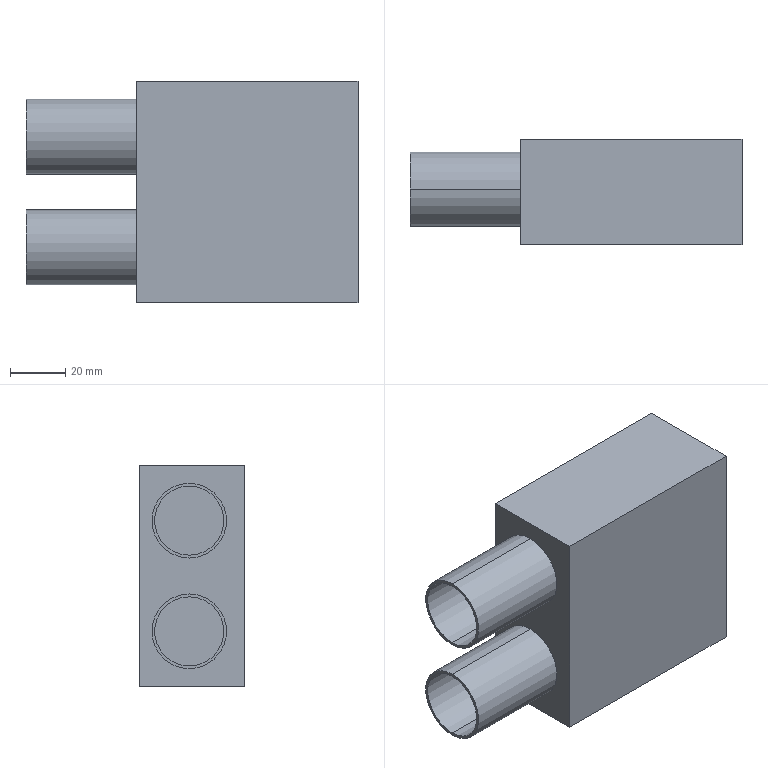Part | SolidWorks | features ICE 2, Cut 1, Extrusion 1 | 1 solid | 21 faces | box 120 x 38 x 80 mm | volume 39835 mm3 | plane 13 | cylinder 8 | commonest cylinder face diameters 25 x4 27 x4
STEP:
#1=CARTESIAN_POINT('',(-80.,20.,33.5));
#2=VERTEX_POINT('',#1);
#3=CARTESIAN_POINT('',(-80.,20.,6.5));
#4=VERTEX_POINT('',#3);
#5=CARTESIAN_POINT('',(-80.,20.,20.));
#6=DIRECTION('',(-1.,0.,0.));
#7=DIRECTION('',(0.,0.,1.));
#8=AXIS2_PLACEMENT_3D('',#5,#6,#7);
#9=CIRCLE('',#8,13.5);
#10=EDGE_CURVE('',#2,#4,#9,.T.);
#11=ORIENTED_EDGE('',*,*,#10,.F.);
#12=CARTESIAN_POINT('',(-40.,20.,33.5));
#13=VERTEX_POINT('',#12);
#14=CARTESIAN_POINT('',(-80.,20.,33.5));
#15=DIRECTION('',(1.,0.,0.));
#16=VECTOR('',#15,1000.);
#17=LINE('',#14,#16);
#18=EDGE_CURVE('',#2,#13,#17,.T.);
#19=ORIENTED_EDGE('',*,*,#18,.T.);
#20=CARTESIAN_POINT('',(-40.,20.,6.5));
#21=VERTEX_POINT('',#20);
#22=CARTESIAN_POINT('',(-40.,20.,20.));
#23=DIRECTION('',(-1.,0.,0.));
#24=DIRECTION('',(0.,0.,-1.));
#25=AXIS2_PLACEMENT_3D('',#22,#23,#24);
#26=CIRCLE('',#25,13.5);
#27=EDGE_CURVE('',#13,#21,#26,.T.);
#28=ORIENTED_EDGE('',*,*,#27,.T.);
#29=CARTESIAN_POINT('',(-80.,20.,6.5));
#30=DIRECTION('',(1.,0.,0.));
#31=VECTOR('',#30,1000.);
#32=LINE('',#29,#31);
#33=EDGE_CURVE('',#4,#21,#32,.T.);
#34=ORIENTED_EDGE('',*,*,#33,.F.);
#35=EDGE_LOOP('',(#11,#19,#28,#34));
#36=FACE_OUTER_BOUND('',#35,.T.);
#37=CARTESIAN_POINT('',(-80.,20.,20.));
#38=DIRECTION('',(1.,0.,0.));
#39=DIRECTION('',(0.,0.,-1.));
#40=AXIS2_PLACEMENT_3D('',#37,#38,#39);
#41=CYLINDRICAL_SURFACE('',#40,13.5);
#42=ADVANCED_FACE('',(#36),#41,.T.);
#43=CARTESIAN_POINT('',(-80.,20.,-6.5));
#44=VERTEX_POINT('',#43);
#45=CARTESIAN_POINT('',(-80.,20.,-33.5));
#46=VERTEX_POINT('',#45);
#47=CARTESIAN_POINT('',(-80.,20.,-20.));
#48=DIRECTION('',(-1.,0.,0.));
#49=DIRECTION('',(0.,0.,1.));
#50=AXIS2_PLACEMENT_3D('',#47,#48,#49);
#51=CIRCLE('',#50,13.5);
#52=EDGE_CURVE('',#44,#46,#51,.T.);
#53=ORIENTED_EDGE('',*,*,#52,.F.);
#54=CARTESIAN_POINT('',(-40.,20.,-6.5));
#55=VERTEX_POINT('',#54);
#56=CARTESIAN_POINT('',(-80.,20.,-6.5));
#57=DIRECTION('',(1.,0.,0.));
#58=VECTOR('',#57,1000.);
#59=LINE('',#56,#58);
#60=EDGE_CURVE('',#44,#55,#59,.T.);
#61=ORIENTED_EDGE('',*,*,#60,.T.);
#62=CARTESIAN_POINT('',(-40.,20.,-33.5));
#63=VERTEX_POINT('',#62);
#64=CARTESIAN_POINT('',(-40.,20.,-20.));
#65=DIRECTION('',(-1.,0.,0.));
#66=DIRECTION('',(0.,0.,-1.));
#67=AXIS2_PLACEMENT_3D('',#64,#65,#66);
#68=CIRCLE('',#67,13.5);
#69=EDGE_CURVE('',#55,#63,#68,.T.);
#70=ORIENTED_EDGE('',*,*,#69,.T.);
#71=CARTESIAN_POINT('',(-80.,20.,-33.5));
#72=DIRECTION('',(1.,0.,0.));
#73=VECTOR('',#72,1000.);
#74=LINE('',#71,#73);
#75=EDGE_CURVE('',#46,#63,#74,.T.);
#76=ORIENTED_EDGE('',*,*,#75,.F.);
#77=EDGE_LOOP('',(#53,#61,#70,#76));
#78=FACE_OUTER_BOUND('',#77,.T.);
#79=CARTESIAN_POINT('',(-80.,20.,-20.));
#80=DIRECTION('',(1.,0.,0.));
#81=DIRECTION('',(0.,0.,-1.));
#82=AXIS2_PLACEMENT_3D('',#79,#80,#81);
#83=CYLINDRICAL_SURFACE('',#82,13.5);
#84=ADVANCED_FACE('',(#78),#83,.T.);
#85=CARTESIAN_POINT('',(-38.,20.,-32.5));
#86=VERTEX_POINT('',#85);
#87=CARTESIAN_POINT('',(-38.,20.,-7.5));
#88=VERTEX_POINT('',#87);
#89=CARTESIAN_POINT('',(-38.,20.,-20.));
#90=DIRECTION('',(-1.,0.,0.));
#91=DIRECTION('',(0.,0.,1.));
#92=AXIS2_PLACEMENT_3D('',#89,#90,#91);
#93=CIRCLE('',#92,12.5);
#94=EDGE_CURVE('',#86,#88,#93,.T.);
#95=ORIENTED_EDGE('',*,*,#94,.F.);
#96=CARTESIAN_POINT('',(-80.,20.,-32.5));
#97=VERTEX_POINT('',#96);
#98=CARTESIAN_POINT('',(-30.,20.,-32.5));
#99=DIRECTION('',(-1.,0.,0.));
#100=VECTOR('',#99,1000.);
#101=LINE('',#98,#100);
#102=EDGE_CURVE('',#86,#97,#101,.T.);
#103=ORIENTED_EDGE('',*,*,#102,.T.);
#104=CARTESIAN_POINT('',(-80.,20.,-7.5));
#105=VERTEX_POINT('',#104);
#106=CARTESIAN_POINT('',(-80.,20.,-20.));
#107=DIRECTION('',(-1.,0.,0.));
#108=DIRECTION('',(0.,0.,1.));
#109=AXIS2_PLACEMENT_3D('',#106,#107,#108);
#110=CIRCLE('',#109,12.5);
#111=EDGE_CURVE('',#97,#105,#110,.T.);
#112=ORIENTED_EDGE('',*,*,#111,.T.);
#113=CARTESIAN_POINT('',(-30.,20.,-7.5));
#114=DIRECTION('',(-1.,0.,0.));
#115=VECTOR('',#114,1000.);
#116=LINE('',#113,#115);
#117=EDGE_CURVE('',#88,#105,#116,.T.);
#118=ORIENTED_EDGE('',*,*,#117,.F.);
#119=EDGE_LOOP('',(#95,#103,#112,#118));
#120=FACE_OUTER_BOUND('',#119,.T.);
#121=CARTESIAN_POINT('',(-30.,20.,-20.));
#122=DIRECTION('',(-1.,0.,0.));
#123=DIRECTION('',(0.,0.,1.));
#124=AXIS2_PLACEMENT_3D('',#121,#122,#123);
#125=CYLINDRICAL_SURFACE('',#124,12.5);
#126=ADVANCED_FACE('',(#120),#125,.F.);
#127=CARTESIAN_POINT('',(-38.,20.,7.5));
#128=VERTEX_POINT('',#127);
#129=CARTESIAN_POINT('',(-38.,20.,32.5));
#130=VERTEX_POINT('',#129);
#131=CARTESIAN_POINT('',(-38.,20.,20.));
#132=DIRECTION('',(-1.,0.,0.));
#133=DIRECTION('',(0.,0.,1.));
#134=AXIS2_PLACEMENT_3D('',#131,#132,#133);
#135=CIRCLE('',#134,12.5);
#136=EDGE_CURVE('',#128,#130,#135,.T.);
#137=ORIENTED_EDGE('',*,*,#136,.F.);
#138=CARTESIAN_POINT('',(-80.,20.,7.5));
#139=VERTEX_POINT('',#138);
#140=CARTESIAN_POINT('',(-30.,20.,7.5));
#141=DIRECTION('',(-1.,0.,0.));
#142=VECTOR('',#141,1000.);
#143=LINE('',#140,#142);
#144=EDGE_CURVE('',#128,#139,#143,.T.);
#145=ORIENTED_EDGE('',*,*,#144,.T.);
#146=CARTESIAN_POINT('',(-80.,20.,32.5));
#147=VERTEX_POINT('',#146);
#148=CARTESIAN_POINT('',(-80.,20.,20.));
#149=DIRECTION('',(-1.,0.,0.));
#150=DIRECTION('',(0.,0.,1.));
#151=AXIS2_PLACEMENT_3D('',#148,#149,#150);
#152=CIRCLE('',#151,12.5);
#153=EDGE_CURVE('',#139,#147,#152,.T.);
#154=ORIENTED_EDGE('',*,*,#153,.T.);
#155=CARTESIAN_POINT('',(-30.,20.,32.5));
#156=DIRECTION('',(-1.,0.,0.));
#157=VECTOR('',#156,1000.);
#158=LINE('',#155,#157);
#159=EDGE_CURVE('',#130,#147,#158,.T.);
#160=ORIENTED_EDGE('',*,*,#159,.F.);
#161=EDGE_LOOP('',(#137,#145,#154,#160));
#162=FACE_OUTER_BOUND('',#161,.T.);
#163=CARTESIAN_POINT('',(-30.,20.,20.));
#164=DIRECTION('',(-1.,0.,0.));
#165=DIRECTION('',(0.,0.,1.));
#166=AXIS2_PLACEMENT_3D('',#163,#164,#165);
#167=CYLINDRICAL_SURFACE('',#166,12.5);
#168=ADVANCED_FACE('',(#162),#167,.F.);
#169=CARTESIAN_POINT('',(-40.,20.,-20.));
#170=DIRECTION('',(-1.,0.,0.));
#171=DIRECTION('',(0.,0.,-1.));
#172=AXIS2_PLACEMENT_3D('',#169,#170,#171);
#173=CIRCLE('',#172,13.5);
#174=EDGE_CURVE('',#63,#55,#173,.T.);
#175=ORIENTED_EDGE('',*,*,#174,.F.);
#176=ORIENTED_EDGE('',*,*,#69,.F.);
#177=EDGE_LOOP('',(#175,#176));
#178=FACE_BOUND('',#177,.T.);
#179=CARTESIAN_POINT('',(-40.,0.,-40.));
#180=VERTEX_POINT('',#179);
#181=CARTESIAN_POINT('',(-40.,0.,40.));
#182=VERTEX_POINT('',#181);
#183=CARTESIAN_POINT('',(-40.,0.,-40.));
#184=DIRECTION('',(0.,0.,1.));
#185=VECTOR('',#184,1000.);
#186=LINE('',#183,#185);
#187=EDGE_CURVE('',#180,#182,#186,.T.);
#188=ORIENTED_EDGE('',*,*,#187,.T.);
#189=CARTESIAN_POINT('',(-40.,38.,40.));
#190=VERTEX_POINT('',#189);
#191=CARTESIAN_POINT('',(-40.,38.,40.));
#192=DIRECTION('',(0.,-1.,0.));
#193=VECTOR('',#192,1000.);
#194=LINE('',#191,#193);
#195=EDGE_CURVE('',#190,#182,#194,.T.);
#196=ORIENTED_EDGE('',*,*,#195,.F.);
#197=CARTESIAN_POINT('',(-40.,38.,-40.));
#198=VERTEX_POINT('',#197);
#199=CARTESIAN_POINT('',(-40.,38.,-40.));
#200=DIRECTION('',(0.,0.,1.));
#201=VECTOR('',#200,1000.);
#202=LINE('',#199,#201);
#203=EDGE_CURVE('',#198,#190,#202,.T.);
#204=ORIENTED_EDGE('',*,*,#203,.F.);
#205=CARTESIAN_POINT('',(-40.,38.,-40.));
#206=DIRECTION('',(0.,-1.,0.));
#207=VECTOR('',#206,1000.);
#208=LINE('',#205,#207);
#209=EDGE_CURVE('',#198,#180,#208,.T.);
#210=ORIENTED_EDGE('',*,*,#209,.T.);
#211=EDGE_LOOP('',(#188,#196,#204,#210));
#212=FACE_OUTER_BOUND('',#211,.T.);
#213=CARTESIAN_POINT('',(-40.,20.,20.));
#214=DIRECTION('',(-1.,0.,0.));
#215=DIRECTION('',(0.,0.,-1.));
#216=AXIS2_PLACEMENT_3D('',#213,#214,#215);
#217=CIRCLE('',#216,13.5);
#218=EDGE_CURVE('',#21,#13,#217,.T.);
#219=ORIENTED_EDGE('',*,*,#218,.F.);
#220=ORIENTED_EDGE('',*,*,#27,.F.);
#221=EDGE_LOOP('',(#219,#220));
#222=FACE_BOUND('',#221,.T.);
#223=CARTESIAN_POINT('',(-40.,38.,-40.));
#224=DIRECTION('',(1.,0.,0.));
#225=DIRECTION('',(0.,0.,-1.));
#226=AXIS2_PLACEMENT_3D('',#223,#224,#225);
#227=PLANE('',#226);
#228=ADVANCED_FACE('',(#178,#212,#222),#227,.F.);
#229=CARTESIAN_POINT('',(40.,0.,40.));
#230=VERTEX_POINT('',#229);
#231=CARTESIAN_POINT('',(40.,0.,-40.));
#232=VERTEX_POINT('',#231);
#233=CARTESIAN_POINT('',(40.,0.,-40.));
#234=DIRECTION('',(0.,0.,-1.));
#235=VECTOR('',#234,1000.);
#236=LINE('',#233,#235);
#237=EDGE_CURVE('',#230,#232,#236,.T.);
#238=ORIENTED_EDGE('',*,*,#237,.T.);
#239=CARTESIAN_POINT('',(40.,38.,-40.));
#240=VERTEX_POINT('',#239);
#241=CARTESIAN_POINT('',(40.,38.,-40.));
#242=DIRECTION('',(0.,-1.,0.));
#243=VECTOR('',#242,1000.);
#244=LINE('',#241,#243);
#245=EDGE_CURVE('',#240,#232,#244,.T.);
#246=ORIENTED_EDGE('',*,*,#245,.F.);
#247=CARTESIAN_POINT('',(40.,38.,40.));
#248=VERTEX_POINT('',#247);
#249=CARTESIAN_POINT('',(40.,38.,-40.));
#250=DIRECTION('',(0.,0.,-1.));
#251=VECTOR('',#250,1000.);
#252=LINE('',#249,#251);
#253=EDGE_CURVE('',#248,#240,#252,.T.);
#254=ORIENTED_EDGE('',*,*,#253,.F.);
#255=CARTESIAN_POINT('',(40.,38.,40.));
#256=DIRECTION('',(0.,-1.,0.));
#257=VECTOR('',#256,1000.);
#258=LINE('',#255,#257);
#259=EDGE_CURVE('',#248,#230,#258,.T.);
#260=ORIENTED_EDGE('',*,*,#259,.T.);
#261=EDGE_LOOP('',(#238,#246,#254,#260));
#262=FACE_OUTER_BOUND('',#261,.T.);
#263=CARTESIAN_POINT('',(40.,38.,-40.));
#264=DIRECTION('',(-1.,0.,0.));
#265=DIRECTION('',(0.,0.,1.));
#266=AXIS2_PLACEMENT_3D('',#263,#264,#265);
#267=PLANE('',#266);
#268=ADVANCED_FACE('',(#262),#267,.F.);
#269=CARTESIAN_POINT('',(-40.,0.,-40.));
#270=DIRECTION('',(-1.,0.,0.));
#271=VECTOR('',#270,1000.);
#272=LINE('',#269,#271);
#273=EDGE_CURVE('',#232,#180,#272,.T.);
#274=ORIENTED_EDGE('',*,*,#273,.T.);
#275=ORIENTED_EDGE('',*,*,#209,.F.);
#276=CARTESIAN_POINT('',(-40.,38.,-40.));
#277=DIRECTION('',(-1.,0.,0.));
#278=VECTOR('',#277,1000.);
#279=LINE('',#276,#278);
#280=EDGE_CURVE('',#240,#198,#279,.T.);
#281=ORIENTED_EDGE('',*,*,#280,.F.);
#282=ORIENTED_EDGE('',*,*,#245,.T.);
#283=EDGE_LOOP('',(#274,#275,#281,#282));
#284=FACE_OUTER_BOUND('',#283,.T.);
#285=CARTESIAN_POINT('',(-40.,38.,-40.));
#286=DIRECTION('',(0.,0.,1.));
#287=DIRECTION('',(1.,0.,0.));
#288=AXIS2_PLACEMENT_3D('',#285,#286,#287);
#289=PLANE('',#288);
#290=ADVANCED_FACE('',(#284),#289,.F.);
#291=CARTESIAN_POINT('',(-40.,0.,40.));
#292=DIRECTION('',(1.,0.,0.));
#293=VECTOR('',#292,1000.);
#294=LINE('',#291,#293);
#295=EDGE_CURVE('',#182,#230,#294,.T.);
#296=ORIENTED_EDGE('',*,*,#295,.T.);
#297=ORIENTED_EDGE('',*,*,#259,.F.);
#298=CARTESIAN_POINT('',(-40.,38.,40.));
#299=DIRECTION('',(1.,0.,0.));
#300=VECTOR('',#299,1000.);
#301=LINE('',#298,#300);
#302=EDGE_CURVE('',#190,#248,#301,.T.);
#303=ORIENTED_EDGE('',*,*,#302,.F.);
#304=ORIENTED_EDGE('',*,*,#195,.T.);
#305=EDGE_LOOP('',(#296,#297,#303,#304));
#306=FACE_OUTER_BOUND('',#305,.T.);
#307=CARTESIAN_POINT('',(-40.,38.,40.));
#308=DIRECTION('',(0.,0.,-1.));
#309=DIRECTION('',(-1.,0.,0.));
#310=AXIS2_PLACEMENT_3D('',#307,#308,#309);
#311=PLANE('',#310);
#312=ADVANCED_FACE('',(#306),#311,.F.);
#313=CARTESIAN_POINT('',(38.,38.,38.));
#314=VERTEX_POINT('',#313);
#315=CARTESIAN_POINT('',(38.,38.,-38.));
#316=VERTEX_POINT('',#315);
#317=CARTESIAN_POINT('',(38.,38.,38.));
#318=DIRECTION('',(0.,0.,-1.));
#319=VECTOR('',#318,1000.);
#320=LINE('',#317,#319);
#321=EDGE_CURVE('',#314,#316,#320,.T.);
#322=ORIENTED_EDGE('',*,*,#321,.F.);
#323=CARTESIAN_POINT('',(-38.,38.,38.));
#324=VERTEX_POINT('',#323);
#325=CARTESIAN_POINT('',(-38.,38.,38.));
#326=DIRECTION('',(1.,0.,0.));
#327=VECTOR('',#326,1000.);
#328=LINE('',#325,#327);
#329=EDGE_CURVE('',#324,#314,#328,.T.);
#330=ORIENTED_EDGE('',*,*,#329,.F.);
#331=CARTESIAN_POINT('',(-38.,38.,-38.));
#332=VERTEX_POINT('',#331);
#333=CARTESIAN_POINT('',(-38.,38.,38.));
#334=DIRECTION('',(0.,0.,1.));
#335=VECTOR('',#334,1000.);
#336=LINE('',#333,#335);
#337=EDGE_CURVE('',#332,#324,#336,.T.);
#338=ORIENTED_EDGE('',*,*,#337,.F.);
#339=CARTESIAN_POINT('',(-38.,38.,-38.));
#340=DIRECTION('',(-1.,0.,0.));
#341=VECTOR('',#340,1000.);
#342=LINE('',#339,#341);
#343=EDGE_CURVE('',#316,#332,#342,.T.);
#344=ORIENTED_EDGE('',*,*,#343,.F.);
#345=EDGE_LOOP('',(#322,#330,#338,#344));
#346=FACE_BOUND('',#345,.T.);
#347=ORIENTED_EDGE('',*,*,#253,.T.);
#348=ORIENTED_EDGE('',*,*,#280,.T.);
#349=ORIENTED_EDGE('',*,*,#203,.T.);
#350=ORIENTED_EDGE('',*,*,#302,.T.);
#351=EDGE_LOOP('',(#347,#348,#349,#350));
#352=FACE_OUTER_BOUND('',#351,.T.);
#353=CARTESIAN_POINT('',(0.,38.,0.));
#354=DIRECTION('',(0.,1.,0.));
#355=DIRECTION('',(0.,0.,1.));
#356=AXIS2_PLACEMENT_3D('',#353,#354,#355);
#357=PLANE('',#356);
#358=ADVANCED_FACE('',(#346,#352),#357,.T.);
#359=ORIENTED_EDGE('',*,*,#237,.F.);
#360=ORIENTED_EDGE('',*,*,#295,.F.);
#361=ORIENTED_EDGE('',*,*,#187,.F.);
#362=ORIENTED_EDGE('',*,*,#273,.F.);
#363=EDGE_LOOP('',(#359,#360,#361,#362));
#364=FACE_OUTER_BOUND('',#363,.T.);
#365=CARTESIAN_POINT('',(0.,0.,0.));
#366=DIRECTION('',(0.,1.,0.));
#367=DIRECTION('',(0.,0.,1.));
#368=AXIS2_PLACEMENT_3D('',#365,#366,#367);
#369=PLANE('',#368);
#370=ADVANCED_FACE('',(#364),#369,.F.);
#371=ORIENTED_EDGE('',*,*,#321,.T.);
#372=CARTESIAN_POINT('',(38.,2.,-38.));
#373=VERTEX_POINT('',#372);
#374=CARTESIAN_POINT('',(38.,2.,-38.));
#375=DIRECTION('',(0.,1.,0.));
#376=VECTOR('',#375,1000.);
#377=LINE('',#374,#376);
#378=EDGE_CURVE('',#373,#316,#377,.T.);
#379=ORIENTED_EDGE('',*,*,#378,.F.);
#380=CARTESIAN_POINT('',(38.,2.,38.));
#381=VERTEX_POINT('',#380);
#382=CARTESIAN_POINT('',(38.,2.,38.));
#383=DIRECTION('',(0.,0.,-1.));
#384=VECTOR('',#383,1000.);
#385=LINE('',#382,#384);
#386=EDGE_CURVE('',#381,#373,#385,.T.);
#387=ORIENTED_EDGE('',*,*,#386,.F.);
#388=CARTESIAN_POINT('',(38.,2.,38.));
#389=DIRECTION('',(0.,1.,0.));
#390=VECTOR('',#389,1000.);
#391=LINE('',#388,#390);
#392=EDGE_CURVE('',#381,#314,#391,.T.);
#393=ORIENTED_EDGE('',*,*,#392,.T.);
#394=EDGE_LOOP('',(#371,#379,#387,#393));
#395=FACE_OUTER_BOUND('',#394,.T.);
#396=CARTESIAN_POINT('',(38.,2.,38.));
#397=DIRECTION('',(1.,0.,0.));
#398=DIRECTION('',(0.,0.,-1.));
#399=AXIS2_PLACEMENT_3D('',#396,#397,#398);
#400=PLANE('',#399);
#401=ADVANCED_FACE('',(#395),#400,.F.);
#402=ORIENTED_EDGE('',*,*,#329,.T.);
#403=ORIENTED_EDGE('',*,*,#392,.F.);
#404=CARTESIAN_POINT('',(-38.,2.,38.));
#405=VERTEX_POINT('',#404);
#406=CARTESIAN_POINT('',(-38.,2.,38.));
#407=DIRECTION('',(1.,0.,0.));
#408=VECTOR('',#407,1000.);
#409=LINE('',#406,#408);
#410=EDGE_CURVE('',#405,#381,#409,.T.);
#411=ORIENTED_EDGE('',*,*,#410,.F.);
#412=CARTESIAN_POINT('',(-38.,2.,38.));
#413=DIRECTION('',(0.,1.,0.));
#414=VECTOR('',#413,1000.);
#415=LINE('',#412,#414);
#416=EDGE_CURVE('',#405,#324,#415,.T.);
#417=ORIENTED_EDGE('',*,*,#416,.T.);
#418=EDGE_LOOP('',(#402,#403,#411,#417));
#419=FACE_OUTER_BOUND('',#418,.T.);
#420=CARTESIAN_POINT('',(-38.,2.,38.));
#421=DIRECTION('',(0.,0.,1.));
#422=DIRECTION('',(1.,0.,0.));
#423=AXIS2_PLACEMENT_3D('',#420,#421,#422);
#424=PLANE('',#423);
#425=ADVANCED_FACE('',(#419),#424,.F.);
#426=CARTESIAN_POINT('',(-38.,20.,-20.));
#427=DIRECTION('',(-1.,0.,0.));
#428=DIRECTION('',(0.,0.,1.));
#429=AXIS2_PLACEMENT_3D('',#426,#427,#428);
#430=CIRCLE('',#429,12.5);
#431=EDGE_CURVE('',#88,#86,#430,.T.);
#432=ORIENTED_EDGE('',*,*,#431,.T.);
#433=ORIENTED_EDGE('',*,*,#94,.T.);
#434=EDGE_LOOP('',(#432,#433));
#435=FACE_BOUND('',#434,.T.);
#436=CARTESIAN_POINT('',(-38.,20.,20.));
#437=DIRECTION('',(-1.,0.,0.));
#438=DIRECTION('',(0.,0.,1.));
#439=AXIS2_PLACEMENT_3D('',#436,#437,#438);
#440=CIRCLE('',#439,12.5);
#441=EDGE_CURVE('',#130,#128,#440,.T.);
#442=ORIENTED_EDGE('',*,*,#441,.T.);
#443=ORIENTED_EDGE('',*,*,#136,.T.);
#444=EDGE_LOOP('',(#442,#443));
#445=FACE_BOUND('',#444,.T.);
#446=ORIENTED_EDGE('',*,*,#337,.T.);
#447=ORIENTED_EDGE('',*,*,#416,.F.);
#448=CARTESIAN_POINT('',(-38.,2.,-38.));
#449=VERTEX_POINT('',#448);
#450=CARTESIAN_POINT('',(-38.,2.,38.));
#451=DIRECTION('',(0.,0.,1.));
#452=VECTOR('',#451,1000.);
#453=LINE('',#450,#452);
#454=EDGE_CURVE('',#449,#405,#453,.T.);
#455=ORIENTED_EDGE('',*,*,#454,.F.);
#456=CARTESIAN_POINT('',(-38.,2.,-38.));
#457=DIRECTION('',(0.,1.,0.));
#458=VECTOR('',#457,1000.);
#459=LINE('',#456,#458);
#460=EDGE_CURVE('',#449,#332,#459,.T.);
#461=ORIENTED_EDGE('',*,*,#460,.T.);
#462=EDGE_LOOP('',(#446,#447,#455,#461));
#463=FACE_OUTER_BOUND('',#462,.T.);
#464=CARTESIAN_POINT('',(-38.,2.,38.));
#465=DIRECTION('',(-1.,0.,0.));
#466=DIRECTION('',(0.,0.,1.));
#467=AXIS2_PLACEMENT_3D('',#464,#465,#466);
#468=PLANE('',#467);
#469=ADVANCED_FACE('',(#435,#445,#463),#468,.F.);
#470=ORIENTED_EDGE('',*,*,#343,.T.);
#471=ORIENTED_EDGE('',*,*,#460,.F.);
#472=CARTESIAN_POINT('',(-38.,2.,-38.));
#473=DIRECTION('',(-1.,0.,0.));
#474=VECTOR('',#473,1000.);
#475=LINE('',#472,#474);
#476=EDGE_CURVE('',#373,#449,#475,.T.);
#477=ORIENTED_EDGE('',*,*,#476,.F.);
#478=ORIENTED_EDGE('',*,*,#378,.T.);
#479=EDGE_LOOP('',(#470,#471,#477,#478));
#480=FACE_OUTER_BOUND('',#479,.T.);
#481=CARTESIAN_POINT('',(-38.,2.,-38.));
#482=DIRECTION('',(0.,0.,-1.));
#483=DIRECTION('',(-1.,0.,0.));
#484=AXIS2_PLACEMENT_3D('',#481,#482,#483);
#485=PLANE('',#484);
#486=ADVANCED_FACE('',(#480),#485,.F.);
#487=ORIENTED_EDGE('',*,*,#386,.T.);
#488=ORIENTED_EDGE('',*,*,#476,.T.);
#489=ORIENTED_EDGE('',*,*,#454,.T.);
#490=ORIENTED_EDGE('',*,*,#410,.T.);
#491=EDGE_LOOP('',(#487,#488,#489,#490));
#492=FACE_OUTER_BOUND('',#491,.T.);
#493=CARTESIAN_POINT('',(0.,2.,0.));
#494=DIRECTION('',(0.,-1.,0.));
#495=DIRECTION('',(0.,0.,-1.));
#496=AXIS2_PLACEMENT_3D('',#493,#494,#495);
#497=PLANE('',#496);
#498=ADVANCED_FACE('',(#492),#497,.F.);
#499=ORIENTED_EDGE('',*,*,#144,.F.);
#500=ORIENTED_EDGE('',*,*,#441,.F.);
#501=ORIENTED_EDGE('',*,*,#159,.T.);
#502=CARTESIAN_POINT('',(-80.,20.,20.));
#503=DIRECTION('',(-1.,0.,0.));
#504=DIRECTION('',(0.,0.,1.));
#505=AXIS2_PLACEMENT_3D('',#502,#503,#504);
#506=CIRCLE('',#505,12.5);
#507=EDGE_CURVE('',#147,#139,#506,.T.);
#508=ORIENTED_EDGE('',*,*,#507,.T.);
#509=EDGE_LOOP('',(#499,#500,#501,#508));
#510=FACE_OUTER_BOUND('',#509,.T.);
#511=CARTESIAN_POINT('',(-30.,20.,20.));
#512=DIRECTION('',(-1.,0.,0.));
#513=DIRECTION('',(0.,0.,1.));
#514=AXIS2_PLACEMENT_3D('',#511,#512,#513);
#515=CYLINDRICAL_SURFACE('',#514,12.5);
#516=ADVANCED_FACE('',(#510),#515,.F.);
#517=ORIENTED_EDGE('',*,*,#102,.F.);
#518=ORIENTED_EDGE('',*,*,#431,.F.);
#519=ORIENTED_EDGE('',*,*,#117,.T.);
#520=CARTESIAN_POINT('',(-80.,20.,-20.));
#521=DIRECTION('',(-1.,0.,0.));
#522=DIRECTION('',(0.,0.,1.));
#523=AXIS2_PLACEMENT_3D('',#520,#521,#522);
#524=CIRCLE('',#523,12.5);
#525=EDGE_CURVE('',#105,#97,#524,.T.);
#526=ORIENTED_EDGE('',*,*,#525,.T.);
#527=EDGE_LOOP('',(#517,#518,#519,#526));
#528=FACE_OUTER_BOUND('',#527,.T.);
#529=CARTESIAN_POINT('',(-30.,20.,-20.));
#530=DIRECTION('',(-1.,0.,0.));
#531=DIRECTION('',(0.,0.,1.));
#532=AXIS2_PLACEMENT_3D('',#529,#530,#531);
#533=CYLINDRICAL_SURFACE('',#532,12.5);
#534=ADVANCED_FACE('',(#528),#533,.F.);
#535=CARTESIAN_POINT('',(-80.,20.,-20.));
#536=DIRECTION('',(-1.,0.,0.));
#537=DIRECTION('',(0.,0.,1.));
#538=AXIS2_PLACEMENT_3D('',#535,#536,#537);
#539=CIRCLE('',#538,13.5);
#540=EDGE_CURVE('',#46,#44,#539,.T.);
#541=ORIENTED_EDGE('',*,*,#540,.T.);
#542=ORIENTED_EDGE('',*,*,#52,.T.);
#543=EDGE_LOOP('',(#541,#542));
#544=FACE_OUTER_BOUND('',#543,.T.);
#545=ORIENTED_EDGE('',*,*,#525,.F.);
#546=ORIENTED_EDGE('',*,*,#111,.F.);
#547=EDGE_LOOP('',(#545,#546));
#548=FACE_BOUND('',#547,.T.);
#549=CARTESIAN_POINT('',(-80.,20.,-20.));
#550=DIRECTION('',(-1.,0.,0.));
#551=DIRECTION('',(0.,0.,1.));
#552=AXIS2_PLACEMENT_3D('',#549,#550,#551);
#553=PLANE('',#552);
#554=ADVANCED_FACE('',(#544,#548),#553,.T.);
#555=ORIENTED_EDGE('',*,*,#60,.F.);
#556=ORIENTED_EDGE('',*,*,#540,.F.);
#557=ORIENTED_EDGE('',*,*,#75,.T.);
#558=ORIENTED_EDGE('',*,*,#174,.T.);
#559=EDGE_LOOP('',(#555,#556,#557,#558));
#560=FACE_OUTER_BOUND('',#559,.T.);
#561=CARTESIAN_POINT('',(-80.,20.,-20.));
#562=DIRECTION('',(1.,0.,0.));
#563=DIRECTION('',(0.,0.,-1.));
#564=AXIS2_PLACEMENT_3D('',#561,#562,#563);
#565=CYLINDRICAL_SURFACE('',#564,13.5);
#566=ADVANCED_FACE('',(#560),#565,.T.);
#567=CARTESIAN_POINT('',(-80.,20.,20.));
#568=DIRECTION('',(-1.,0.,0.));
#569=DIRECTION('',(0.,0.,1.));
#570=AXIS2_PLACEMENT_3D('',#567,#568,#569);
#571=CIRCLE('',#570,13.5);
#572=EDGE_CURVE('',#4,#2,#571,.T.);
#573=ORIENTED_EDGE('',*,*,#572,.T.);
#574=ORIENTED_EDGE('',*,*,#10,.T.);
#575=EDGE_LOOP('',(#573,#574));
#576=FACE_OUTER_BOUND('',#575,.T.);
#577=ORIENTED_EDGE('',*,*,#507,.F.);
#578=ORIENTED_EDGE('',*,*,#153,.F.);
#579=EDGE_LOOP('',(#577,#578));
#580=FACE_BOUND('',#579,.T.);
#581=CARTESIAN_POINT('',(-80.,20.,20.));
#582=DIRECTION('',(-1.,0.,0.));
#583=DIRECTION('',(0.,0.,1.));
#584=AXIS2_PLACEMENT_3D('',#581,#582,#583);
#585=PLANE('',#584);
#586=ADVANCED_FACE('',(#576,#580),#585,.T.);
#587=ORIENTED_EDGE('',*,*,#18,.F.);
#588=ORIENTED_EDGE('',*,*,#572,.F.);
#589=ORIENTED_EDGE('',*,*,#33,.T.);
#590=ORIENTED_EDGE('',*,*,#218,.T.);
#591=EDGE_LOOP('',(#587,#588,#589,#590));
#592=FACE_OUTER_BOUND('',#591,.T.);
#593=CARTESIAN_POINT('',(-80.,20.,20.));
#594=DIRECTION('',(1.,0.,0.));
#595=DIRECTION('',(0.,0.,-1.));
#596=AXIS2_PLACEMENT_3D('',#593,#594,#595);
#597=CYLINDRICAL_SURFACE('',#596,13.5);
#598=ADVANCED_FACE('',(#592),#597,.T.);
#599=CLOSED_SHELL('',(#42,#84,#126,#168,#228,#268,#290,#312,#358,#370,#401,#425,#469,#486,#498,#516,#534,#554,#566,#586,#598));
#600=MANIFOLD_SOLID_BREP('',#599);
#601=CARTESIAN_POINT('',(0.,0.,0.));
#602=DIRECTION('',(0.,0.,1.));
#603=DIRECTION('',(1.,0.,0.));
#604=AXIS2_PLACEMENT_3D('',#601,#602,#603);
#605=(LENGTH_UNIT()NAMED_UNIT(*)SI_UNIT(.MILLI.,.METRE.));
#606=UNCERTAINTY_MEASURE_WITH_UNIT(LENGTH_MEASURE(0.00001),#605,'','');
#607=(NAMED_UNIT(*)PLANE_ANGLE_UNIT()SI_UNIT($,.RADIAN.));
#608=(NAMED_UNIT(*)SI_UNIT($,.STERADIAN.)SOLID_ANGLE_UNIT());
#609=(GEOMETRIC_REPRESENTATION_CONTEXT(3)GLOBAL_UNCERTAINTY_ASSIGNED_CONTEXT((#606))GLOBAL_UNIT_ASSIGNED_CONTEXT((#605,#607,#608))REPRESENTATION_CONTEXT('',''));
#610=ADVANCED_BREP_SHAPE_REPRESENTATION('',(#600,#604),#609);